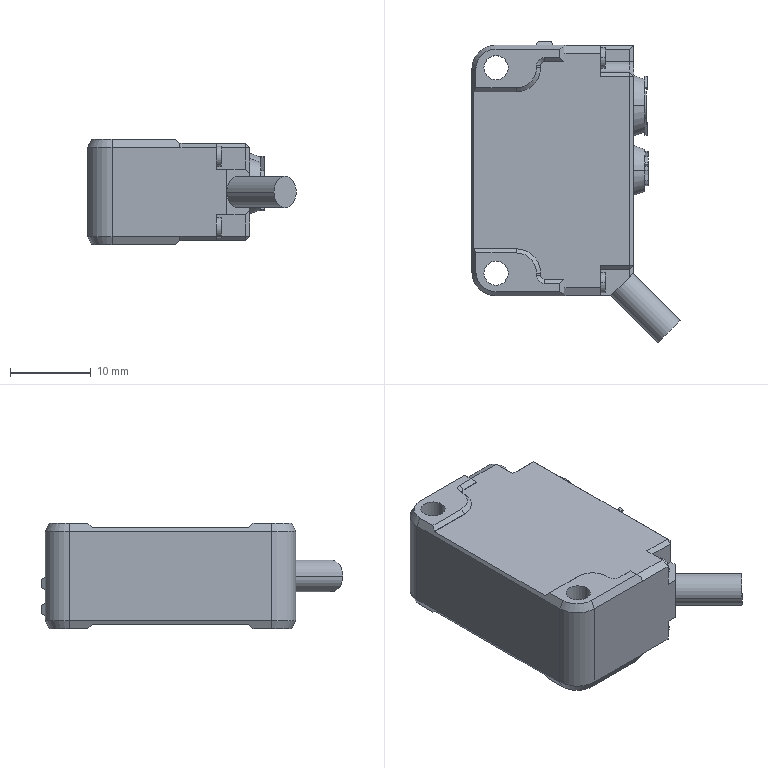Part | SolidWorks | features BaseBody 1 | 1 solid | 251 faces | box 25.77 x 37.32 x 13.1 mm | volume 7336 mm3 | plane 135 | cylinder 99 | cone 17 | commonest cylinder face diameters 0.3 x25 0.5 x22 3.78 x7 2.5 x6 6 x6 0.2 x5